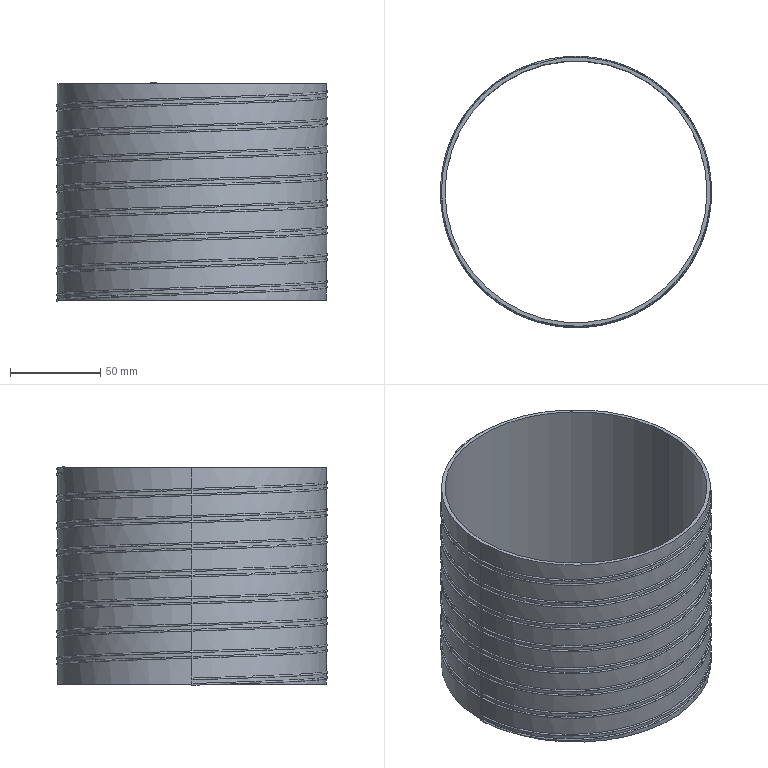Part | STEP file | D1450002 | 1 solid | 43 faces | box 150 x 150 x 121 mm | volume 113645 mm3 | cylinder 33 | plane 6 | spline 4 | commonest cylinder face diameters 149 x31 145 x2